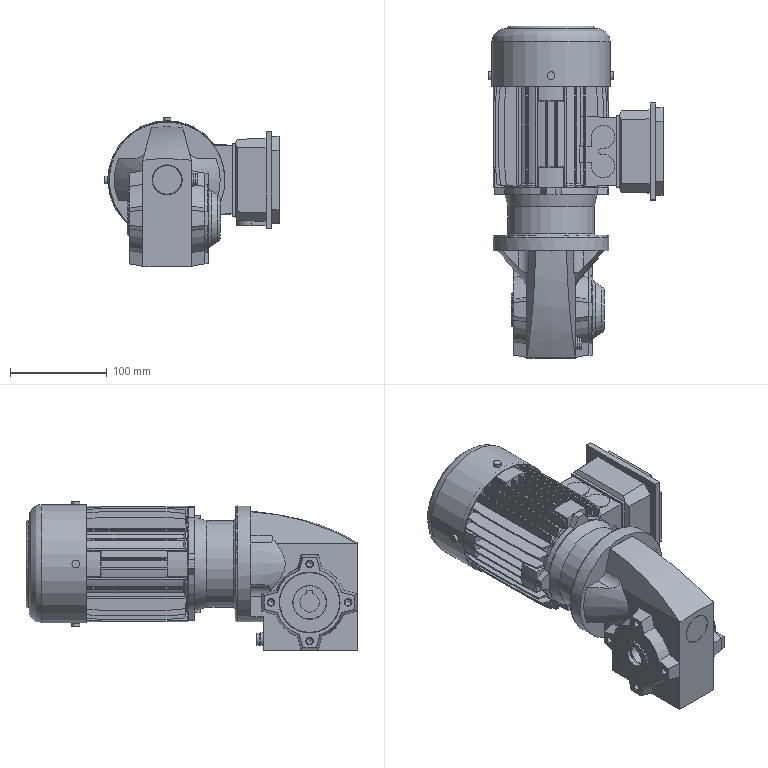Part | STEP file | SK1SMI40AZH-IEC63-63L(1) | 5 solids | 951 faces | box 181.38 x 343.8 x 154.88 mm | volume 3328871 mm3 | plane 564 | cylinder 269 | cone 94 | torus 23 | spline 1 | commonest cylinder face diameters 94.5 x32 24.804 x20 83.121 x20 98 x16 6.4 x10 33.098 x10